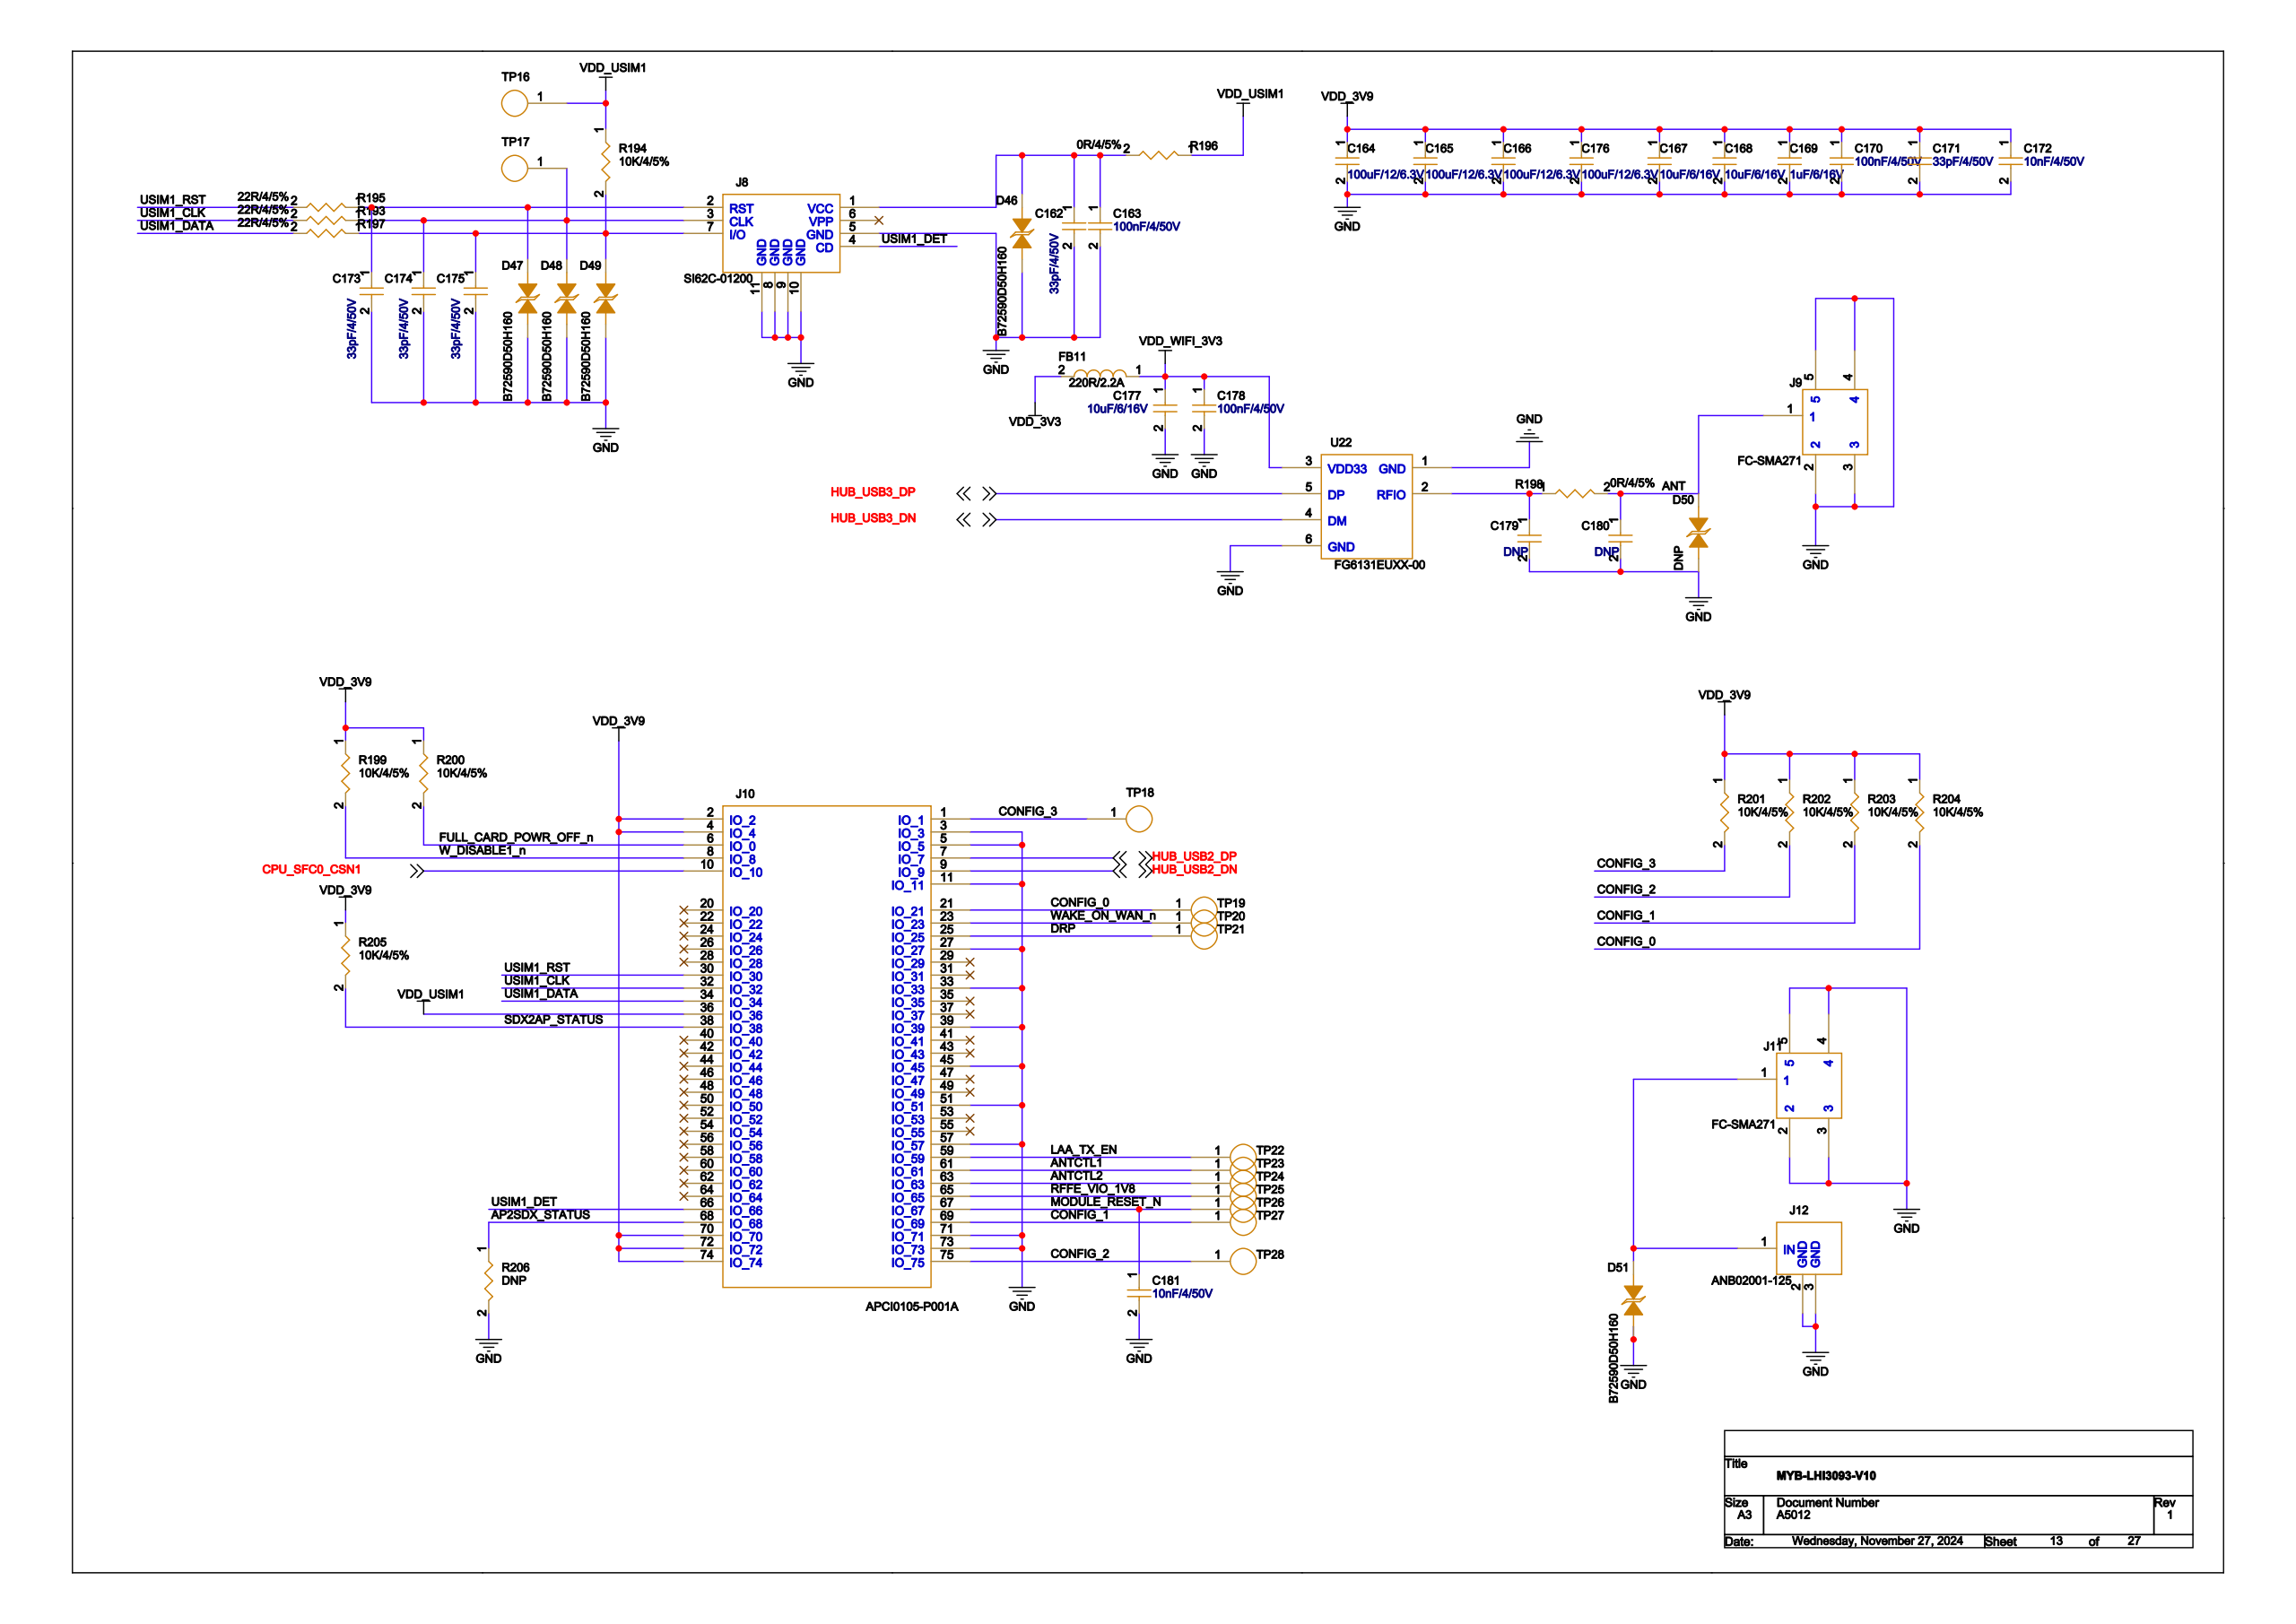Circuit board | Cadence Allegro | 1159 parts | 708 nets | one sheet of the schematic
Parts on this sheet (reference | value | footprint):
C163 | 100nF/4/50V | C0402
C164 | 100uF/12/6.3V | C1206
C165 | 100uF/12/6.3V | C1206
C166 | 100uF/12/6.3V | C1206
C167 | 10uF/6/16V | C0603
C168 | 10uF/6/16V | C0603
C169 | 1uF/6/16V | C0603
C170 | 100nF/4/50V | C0402
C171 | 33pF/4/50V | C0402
C172 | 10nF/4/50V | C0402
C176 | 100uF/12/6.3V | C1206
C177 | 10uF/6/16V | C0603
C178 | 100nF/4/50V | C0402
C179 | DNP | C0402
C180 | DNP | C0402
C181 | 10nF/4/50V | C0402
FB11 | 220R/2.2A | FB0603
J8 | SI62C-01200 | SIM-SI62C-01200
J9 | FC-SMA271 | ANT-5PINS
J10 | APCI0105-P001A | CONN-2199230-3
J11 | FC-SMA271 | ANT-5PINS
J12 | ANB02001-125 | ANT-1566230-1
R194 | 10K/4/5% | R0402
R199 | 10K/4/5% | R0402
R200 | 10K/4/5% | R0402
R201 | 10K/4/5% | R0402
R202 | 10K/4/5% | R0402
R203 | 10K/4/5% | R0402
R204 | 10K/4/5% | R0402
R205 | 10K/4/5% | R0402
R206 | DNP | R0402
TP16 | TP | TPAD_020
TP17 | TP | TPAD_020
TP18 | TP | TPAD_020
TP19 | TP | TPAD_020
TP20 | TP | TPAD_020
TP21 | TP | TPAD_020
TP22 | TP | TPAD_020
TP23 | TP | TPAD_020
TP24 | TP | TPAD_020
TP25 | TP | TPAD_020
TP26 | TP | TPAD_020
TP27 | TP | TPAD_020
TP28 | TP | TPAD_020
U22 | FG6131EUXX-00 | MODILE-FG6188EUFX-05
Nets of these parts (net: part-pin ...):
GND: C163-2 C164-2 C165-2 C166-2 C167-2 C168-2 C169-2 C170-2 C171-2 C172-2 C176-2 C177-2 C178-2 C179-2 C180-2 C181-2 J8-5 J8-8 J8-9 J8-10 J8-11 J9-2 J9-3 J9-4 J9-5 J11-2 J11-3 J11-4 J11-5 J12-2 J12-3 R206-2 U22-1 U22-6 J10-3 J10-5 J10-11 J10-27 J10-33 J10-39 J10-45 J10-51 J10-57 J10-71 J10-73
VDD_3V9: C164-1 C165-1 C166-1 C167-1 C168-1 C169-1 C170-1 C171-1 C172-1 C176-1 R199-1 R200-1 R201-1 R202-1 R203-1 R204-1 R205-1 J10-2 J10-4 J10-70 J10-72 J10-74
VDD_3V3: FB11-2
N14961789: C163-1 J8-1
VDD_WIFI_3V3: C177-1 C178-1 FB11-1 U22-3
N14962558: C179-1 U22-2
ANT: C180-1 J9-1
N14960565: J8-2
N14960569: J8-3 TP17-1
N14960573: J8-7 R194-2
MODULE_RESET_N: C181-1 TP26-1 J10-67
N14964581: J11-1 J12-1
CONFIG_3: R201-2 TP18-1 J10-1
CPU_SFC0_CSN1: J10-10
CONFIG_0: R204-2 TP19-1 J10-21
WAKE_ON_WAN_N: TP20-1 J10-23
DRP: TP21-1 J10-25
USIM1_RST: J10-30
USIM1_CLK: J10-32
USIM1_DATA: J10-34
VDD_USIM1: R194-1 TP16-1 J10-36
SDX2AP_STATUS: R205-2 J10-38
LAA_TX_EN: TP22-1 J10-59
FULL_CARD_POWR_OFF_N: R200-2 J10-6
ANTCTL1: TP23-1 J10-61
ANTCTL2: TP24-1 J10-63
RFFE_VIO_1V8: TP25-1 J10-65
USIM1_DET: J8-4 J10-66
AP2SDX_STATUS: R206-1 J10-68
CONFIG_1: R203-2 TP27-1 J10-69
HUB_USB2_DP: J10-7
CONFIG_2: R202-2 TP28-1 J10-75
W_DISABLE1_N: R199-2 J10-8
HUB_USB2_DN: J10-9
HUB_USB3_DN: U22-4
HUB_USB3_DP: U22-5